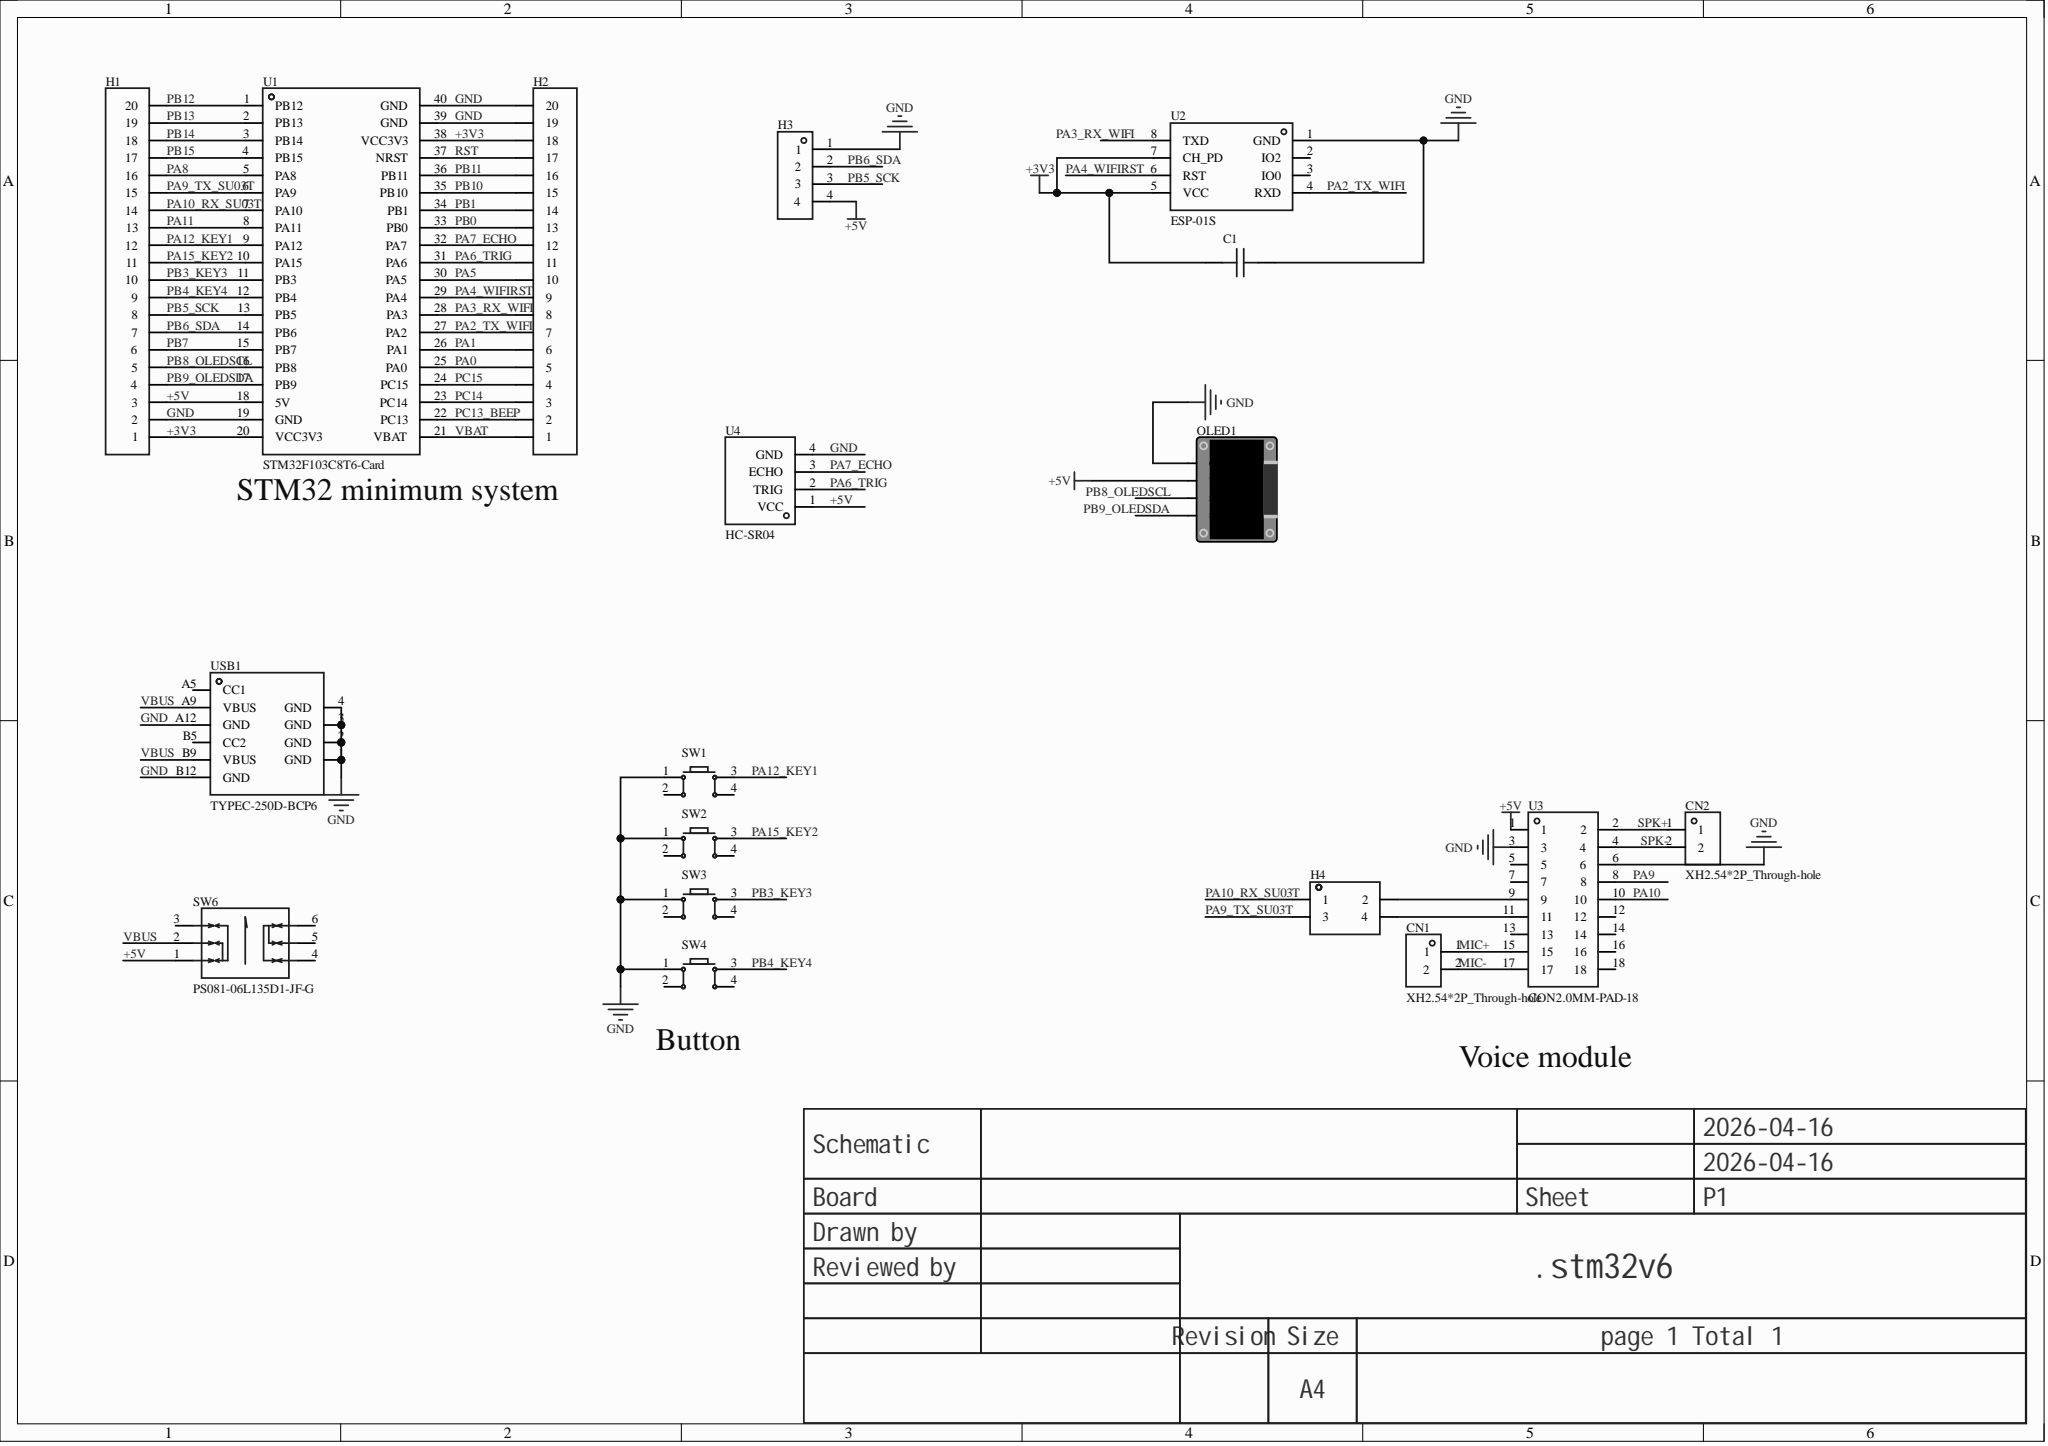Circuit board | Altium Designer | 18 parts | 44 nets
Bill of materials:
Comment,Description,Designator,Footprint,LibRef,Quantity
"100nF","","C1","C0603","CAP_0603","1"
"XH2.54*2P_Through-hole","","CN1, CN2","CONN-TH_2P-P2.50-XH2.54-2P","XH2.54*2P_直插","2"
"","","H1, H2","HDR-TH_20P-P2.54-V-F","HDR-F_2.54_1x20P","2"
"","","H3","HDR-TH_4P-P2.54-V-F","HDR-F_2.54_1x4P","1"
"","","H4","HDR-TH_4P-P2.54-V-F-R2-C2-S2.54","HDR-F_2.54_2x2","1"
"","","OLED1","0.96OLED_4P","0.96OLED模块_4P","1"
"","","SW1, SW2, SW3, SW4","SW-TH_4P-L6.0-W6.0-P4.50-LS6.5","Key_TH_6x6x6","4"
"PS081-06L135D1-JF-G","Circuit structure: DPDT; self-lock/no-lock: self-lock; mounting: through-hole; contact current: 100mA; rated voltage: 30V;","SW6","SW-TH_6P-L8.0-W8.0-P2.50-TL","PS081-06L135D1-JF-G","1"
"STM32F103C8T6-Card","","U1","CONN-TH_L53.3-W22.9_STM32F103C8T6-CARD","STM32F103C8T6-Card","1"
"ESP-01S","","U2","WIFIM-TH_ESP-01S","ESP-01S_C111009","1"
"CON2.0MM-PAD-18","","U3","CONN-TH_18P-P2.00_C9900078766","CON2.0MM-PAD-18","1"
"HC-SR04","","U4","TH_HC-SR04V","HC-SR04","1"
"TYPEC-250D-BCP6","Connector type: Type-C; standard: USB 3.1; gender: female; number of ports: 1; number of contacts: 6P; mounting: SMD flat; rated current - power: 3A; operating temperature range: -25℃~+85℃; soldering temperature (max): 260℃;","USB1","USB-C-SMD_TYPEC-250D-BCP6","TYPEC-250D-BCP6","1"
Netlist (Protel format):
[
C1
C0603
100nF



]
[
CN1
CONN-TH_2P-P2.50-XH2.54-2P
XH2.54*2P_Through-hole



]
[
CN2
CONN-TH_2P-P2.50-XH2.54-2P
XH2.54*2P_Through-hole



]
[
H1
HDR-TH_20P-P2.54-V-F




]
[
H2
HDR-TH_20P-P2.54-V-F




]
[
H3
HDR-TH_4P-P2.54-V-F




]
[
H4
HDR-TH_4P-P2.54-V-F-R2-C2-S2.54




]
[
OLED1
0.96OLED_4P




]
[
SW1
SW-TH_4P-L6.0-W6.0-P4.50-LS6.5




]
[
SW2
SW-TH_4P-L6.0-W6.0-P4.50-LS6.5




]
[
SW3
SW-TH_4P-L6.0-W6.0-P4.50-LS6.5




]
[
SW4
SW-TH_4P-L6.0-W6.0-P4.50-LS6.5




]
[
SW6
SW-TH_6P-L8.0-W8.0-P2.50-TL
PS081-06L135D1-JF-G



]
[
U1
CONN-TH_L53.3-W22.9_STM32F103C8T6-CARD
STM32F103C8T6-Card



]
[
U2
WIFIM-TH_ESP-01S
ESP-01S



]
[
U3
CONN-TH_18P-P2.00_C9900078766
CON2.0MM-PAD-18



]
[
U4
TH_HC-SR04V
HC-SR04



]
[
USB1
USB-C-SMD_TYPEC-250D-BCP6
TYPEC-250D-BCP6



]
(
VBUS
SW6-2
USB1-A9
USB1-B9
)
(
VBAT
H2-1
U1-21
)
(
SPK-
CN2-2
U3-4
)
(
SPK+
CN2-1
U3-2
)
(
RST
H2-17
U1-37
)
(
PC15
H2-4
U1-24
)
(
PC14
H2-3
U1-23
)
(
PC13_BEEP
H2-2
U1-22
)
(
PB15
H1-17
U1-4
)
(
PB14
H1-18
U1-3
)
(
PB13
H1-19
U1-2
)
(
PB12
H1-20
U1-1
)
(
PB11
H2-16
U1-36
)
(
PB10
H2-15
U1-35
)
(
PB9_OLEDSDA
H1-4
OLED1-4
U1-17
)
(
PB8_OLEDSCL
H1-5
OLED1-3
U1-16
)
(
PB7
H1-6
U1-15
)
(
PB6_SDA
H1-7
H3-2
U1-14
)
(
PB5_SCK
H1-8
H3-3
U1-13
)
(
PB4_KEY4
H1-9
SW4-3
U1-12
)
(
PB3_KEY3
H1-10
SW3-3
U1-11
)
(
PB1
H2-14
U1-34
)
(
PB0
H2-13
U1-33
)
(
PA15_KEY2
H1-11
SW2-3
U1-10
)
(
PA12_KEY1
H1-12
SW1-3
U1-9
)
(
PA11
H1-13
U1-8
)
(
PA10_RX_SU03T
H1-14
H4-1
U1-7
)
(
PA9_TX_SU03T
H1-15
H4-3
U1-6
)
(
PA8
H1-16
U1-5
)
(
PA7_ECHO
H2-12
U1-32
U4-3
)
(
PA6_TRIG
H2-11
U1-31
U4-2
)
(
PA5
H2-10
U1-30
)
(
PA4_WIFIRST
H2-9
U1-29
U2-6
)
(
PA3_RX_WIFI
H2-8
U1-28
U2-8
)
(
PA2_TX_WIFI
H2-7
U1-27
U2-4
)
(
PA1
H2-6
U1-26
)
(
PA0
H2-5
U1-25
)
(
NetH4_4
H4-4
U3-11
)
(
NetH4_2
H4-2
U3-9
)
(
MIC-
CN1-2
U3-17
)
(
MIC+
CN1-1
U3-15
)
(
GND
C1-2
H1-2
H2-19
H2-20
H3-1
OLED1-1
SW1-1
SW2-1
SW3-1
SW4-1
U1-19
U1-39
U1-40
U2-1
U3-3
U3-6
U4-4
USB1-1
USB1-2
USB1-3
USB1-4
USB1-A12
USB1-B12
)
(
+5V
H1-3
H3-4
OLED1-2
SW6-1
U1-18
U3-1
U4-1
)
(
+3V3
C1-1
H1-1
H2-18
U1-20
U1-38
U2-5
U2-7
)